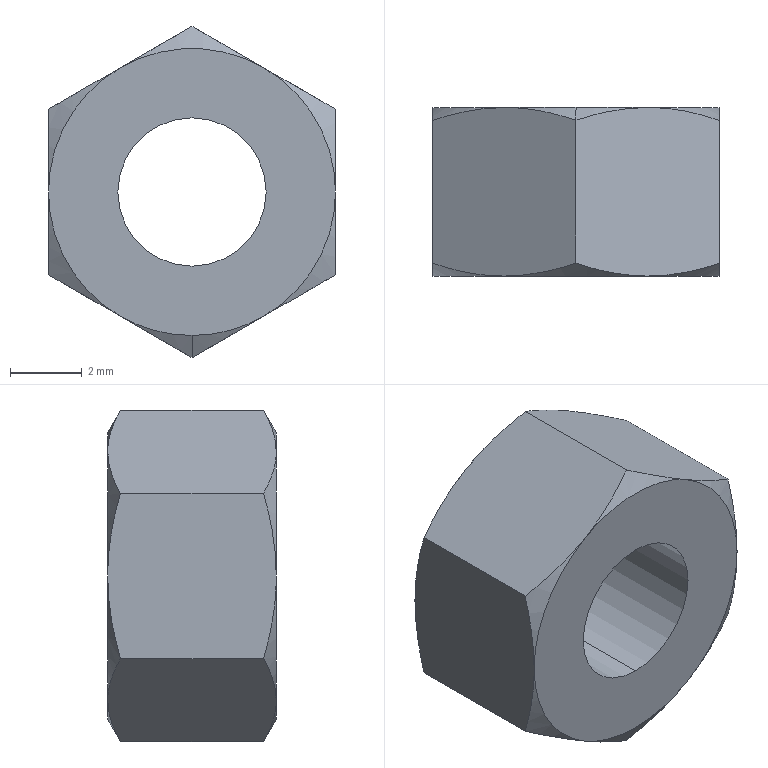Part | STEP file | 1 solid | 24 faces | box 8 x 4.7 x 9.238 mm | volume 196.298 mm3 | cone 14 | plane 8 | cylinder 2 | commonest cylinder face diameters 4.134 x2
STEP:
#1=CARTESIAN_POINT('',(2.,0.,-3.464));
#2=VERTEX_POINT('',#1);
#3=CARTESIAN_POINT('',(0.,0.,-4.));
#4=VERTEX_POINT('',#3);
#5=CARTESIAN_POINT('',(0.,0.,0.));
#6=DIRECTION('',(0.,1.,0.));
#7=DIRECTION('',(0.,0.,1.));
#8=AXIS2_PLACEMENT_3D('',#5,#6,#7);
#9=CIRCLE('',#8,4.);
#10=EDGE_CURVE('',#2,#4,#9,.T.);
#11=ORIENTED_EDGE('',*,*,#10,.T.);
#12=CARTESIAN_POINT('',(0.,0.3573,-4.619));
#13=VERTEX_POINT('',#12);
#14=CARTESIAN_POINT('',(0.,0.,-4.));
#15=DIRECTION('',(0.,0.5,-0.866));
#16=VECTOR('',#15,1000.);
#17=LINE('',#14,#16);
#18=EDGE_CURVE('',#4,#13,#17,.T.);
#19=ORIENTED_EDGE('',*,*,#18,.T.);
#20=CARTESIAN_POINT('',(0.,0.3573,-4.619));
#21=CARTESIAN_POINT('',(0.6543,0.1392,-4.241));
#22=CARTESIAN_POINT('',(1.319,0.,-3.858));
#23=CARTESIAN_POINT('',(2.,0.,-3.464));
#24=B_SPLINE_CURVE_WITH_KNOTS('',3,(#20,#21,#22,#23),.UNSPECIFIED.,.F.,.F.,(4,4),(0.000000238,0.002337),.UNSPECIFIED.);
#25=EDGE_CURVE('',#13,#2,#24,.T.);
#26=ORIENTED_EDGE('',*,*,#25,.T.);
#27=EDGE_LOOP('',(#11,#19,#26));
#28=FACE_OUTER_BOUND('',#27,.T.);
#29=CARTESIAN_POINT('',(0.,0.,0.));
#30=DIRECTION('',(0.,1.,0.));
#31=DIRECTION('',(0.,0.,-1.));
#32=AXIS2_PLACEMENT_3D('',#29,#30,#31);
#33=CONICAL_SURFACE('',#32,4.,1.047);
#34=ADVANCED_FACE('',(#28),#33,.T.);
#35=CARTESIAN_POINT('',(0.,4.7,4.));
#36=VERTEX_POINT('',#35);
#37=CARTESIAN_POINT('',(2.,4.7,3.464));
#38=VERTEX_POINT('',#37);
#39=CARTESIAN_POINT('',(0.,4.7,0.));
#40=DIRECTION('',(0.,1.,0.));
#41=DIRECTION('',(0.,0.,1.));
#42=AXIS2_PLACEMENT_3D('',#39,#40,#41);
#43=CIRCLE('',#42,4.);
#44=EDGE_CURVE('',#36,#38,#43,.T.);
#45=ORIENTED_EDGE('',*,*,#44,.F.);
#46=CARTESIAN_POINT('',(0.,4.343,4.619));
#47=VERTEX_POINT('',#46);
#48=CARTESIAN_POINT('',(0.,4.7,4.));
#49=DIRECTION('',(0.,-0.5,0.866));
#50=VECTOR('',#49,1000.);
#51=LINE('',#48,#50);
#52=EDGE_CURVE('',#36,#47,#51,.T.);
#53=ORIENTED_EDGE('',*,*,#52,.T.);
#54=CARTESIAN_POINT('',(0.,4.343,4.619));
#55=CARTESIAN_POINT('',(0.6543,4.561,4.241));
#56=CARTESIAN_POINT('',(1.319,4.7,3.858));
#57=CARTESIAN_POINT('',(2.,4.7,3.464));
#58=B_SPLINE_CURVE_WITH_KNOTS('',3,(#54,#55,#56,#57),.UNSPECIFIED.,.F.,.F.,(4,4),(0.000000238,0.002337),.UNSPECIFIED.);
#59=EDGE_CURVE('',#47,#38,#58,.T.);
#60=ORIENTED_EDGE('',*,*,#59,.T.);
#61=EDGE_LOOP('',(#45,#53,#60));
#62=FACE_OUTER_BOUND('',#61,.T.);
#63=CARTESIAN_POINT('',(0.,4.7,0.));
#64=DIRECTION('',(0.,-1.,0.));
#65=DIRECTION('',(0.,0.,1.));
#66=AXIS2_PLACEMENT_3D('',#63,#64,#65);
#67=CONICAL_SURFACE('',#66,4.,1.047);
#68=ADVANCED_FACE('',(#62),#67,.T.);
#69=CARTESIAN_POINT('',(0.,4.7,-2.067));
#70=VERTEX_POINT('',#69);
#71=CARTESIAN_POINT('',(0.,4.7,2.067));
#72=VERTEX_POINT('',#71);
#73=CARTESIAN_POINT('',(0.,4.7,0.));
#74=DIRECTION('',(0.,1.,0.));
#75=DIRECTION('',(0.,0.,1.));
#76=AXIS2_PLACEMENT_3D('',#73,#74,#75);
#77=CIRCLE('',#76,2.067);
#78=EDGE_CURVE('',#70,#72,#77,.T.);
#79=ORIENTED_EDGE('',*,*,#78,.T.);
#80=CARTESIAN_POINT('',(0.,0.,2.067));
#81=VERTEX_POINT('',#80);
#82=CARTESIAN_POINT('',(0.,4.7,2.067));
#83=DIRECTION('',(0.,-1.,0.));
#84=VECTOR('',#83,1000.);
#85=LINE('',#82,#84);
#86=EDGE_CURVE('',#72,#81,#85,.T.);
#87=ORIENTED_EDGE('',*,*,#86,.T.);
#88=CARTESIAN_POINT('',(0.,0.,-2.067));
#89=VERTEX_POINT('',#88);
#90=CARTESIAN_POINT('',(0.,0.,0.));
#91=DIRECTION('',(0.,1.,0.));
#92=DIRECTION('',(0.,0.,1.));
#93=AXIS2_PLACEMENT_3D('',#90,#91,#92);
#94=CIRCLE('',#93,2.067);
#95=EDGE_CURVE('',#89,#81,#94,.T.);
#96=ORIENTED_EDGE('',*,*,#95,.F.);
#97=CARTESIAN_POINT('',(0.,4.7,-2.067));
#98=DIRECTION('',(0.,-1.,0.));
#99=VECTOR('',#98,1000.);
#100=LINE('',#97,#99);
#101=EDGE_CURVE('',#70,#89,#100,.T.);
#102=ORIENTED_EDGE('',*,*,#101,.F.);
#103=EDGE_LOOP('',(#79,#87,#96,#102));
#104=FACE_OUTER_BOUND('',#103,.T.);
#105=CARTESIAN_POINT('',(0.,4.7,0.));
#106=DIRECTION('',(0.,-1.,0.));
#107=DIRECTION('',(0.,0.,-1.));
#108=AXIS2_PLACEMENT_3D('',#105,#106,#107);
#109=CYLINDRICAL_SURFACE('',#108,2.067);
#110=ADVANCED_FACE('',(#104),#109,.F.);
#111=CARTESIAN_POINT('',(-4.,0.3573,-2.309));
#112=VERTEX_POINT('',#111);
#113=CARTESIAN_POINT('',(-2.,0.,-3.464));
#114=VERTEX_POINT('',#113);
#115=CARTESIAN_POINT('',(-4.,0.3573,-2.309));
#116=CARTESIAN_POINT('',(-3.346,0.1392,-2.687));
#117=CARTESIAN_POINT('',(-2.681,0.,-3.071));
#118=CARTESIAN_POINT('',(-2.,0.,-3.464));
#119=B_SPLINE_CURVE_WITH_KNOTS('',3,(#115,#116,#117,#118),.UNSPECIFIED.,.F.,.F.,(4,4),(0.000000238,0.002337),.UNSPECIFIED.);
#120=EDGE_CURVE('',#112,#114,#119,.T.);
#121=ORIENTED_EDGE('',*,*,#120,.F.);
#122=CARTESIAN_POINT('',(-4.,4.343,-2.309));
#123=VERTEX_POINT('',#122);
#124=CARTESIAN_POINT('',(-4.,4.7,-2.309));
#125=DIRECTION('',(0.,-1.,0.));
#126=VECTOR('',#125,1000.);
#127=LINE('',#124,#126);
#128=EDGE_CURVE('',#123,#112,#127,.T.);
#129=ORIENTED_EDGE('',*,*,#128,.F.);
#130=CARTESIAN_POINT('',(-2.,4.7,-3.464));
#131=VERTEX_POINT('',#130);
#132=CARTESIAN_POINT('',(-2.,4.7,-3.464));
#133=CARTESIAN_POINT('',(-2.339,4.7,-3.268));
#134=CARTESIAN_POINT('',(-2.678,4.666,-3.072));
#135=CARTESIAN_POINT('',(-3.345,4.541,-2.688));
#136=CARTESIAN_POINT('',(-3.674,4.452,-2.498));
#137=CARTESIAN_POINT('',(-4.,4.343,-2.309));
#138=B_SPLINE_CURVE_WITH_KNOTS('',3,(#132,#133,#134,#135,#136,#137),.UNSPECIFIED.,.F.,.F.,(4,2,4),(0.002337,0.003501,0.004665),.UNSPECIFIED.);
#139=EDGE_CURVE('',#131,#123,#138,.T.);
#140=ORIENTED_EDGE('',*,*,#139,.F.);
#141=CARTESIAN_POINT('',(0.,4.343,-4.619));
#142=VERTEX_POINT('',#141);
#143=CARTESIAN_POINT('',(0.,4.343,-4.619));
#144=CARTESIAN_POINT('',(-0.6543,4.561,-4.241));
#145=CARTESIAN_POINT('',(-1.319,4.7,-3.858));
#146=CARTESIAN_POINT('',(-2.,4.7,-3.464));
#147=B_SPLINE_CURVE_WITH_KNOTS('',3,(#143,#144,#145,#146),.UNSPECIFIED.,.F.,.F.,(4,4),(0.000000238,0.002337),.UNSPECIFIED.);
#148=EDGE_CURVE('',#142,#131,#147,.T.);
#149=ORIENTED_EDGE('',*,*,#148,.F.);
#150=CARTESIAN_POINT('',(0.,4.7,-4.619));
#151=DIRECTION('',(0.,-1.,0.));
#152=VECTOR('',#151,1000.);
#153=LINE('',#150,#152);
#154=EDGE_CURVE('',#142,#13,#153,.T.);
#155=ORIENTED_EDGE('',*,*,#154,.T.);
#156=CARTESIAN_POINT('',(-2.,0.,-3.464));
#157=CARTESIAN_POINT('',(-1.661,0.,-3.66));
#158=CARTESIAN_POINT('',(-1.322,0.03421,-3.856));
#159=CARTESIAN_POINT('',(-0.6554,0.1587,-4.24));
#160=CARTESIAN_POINT('',(-0.3264,0.2485,-4.43));
#161=CARTESIAN_POINT('',(0.,0.3573,-4.619));
#162=B_SPLINE_CURVE_WITH_KNOTS('',3,(#156,#157,#158,#159,#160,#161),.UNSPECIFIED.,.F.,.F.,(4,2,4),(0.002337,0.003501,0.004665),.UNSPECIFIED.);
#163=EDGE_CURVE('',#114,#13,#162,.T.);
#164=ORIENTED_EDGE('',*,*,#163,.F.);
#165=EDGE_LOOP('',(#121,#129,#140,#149,#155,#164));
#166=FACE_OUTER_BOUND('',#165,.T.);
#167=CARTESIAN_POINT('',(0.,4.7,-4.619));
#168=DIRECTION('',(0.5,0.,0.866));
#169=DIRECTION('',(0.866,0.,-0.5));
#170=AXIS2_PLACEMENT_3D('',#167,#168,#169);
#171=PLANE('',#170);
#172=ADVANCED_FACE('',(#166),#171,.F.);
#173=CARTESIAN_POINT('',(-4.,0.3573,2.309));
#174=VERTEX_POINT('',#173);
#175=CARTESIAN_POINT('',(-4.,0.,0.));
#176=VERTEX_POINT('',#175);
#177=CARTESIAN_POINT('',(-4.,0.3573,2.309));
#178=CARTESIAN_POINT('',(-4.,0.2494,1.936));
#179=CARTESIAN_POINT('',(-4.,0.1597,1.558));
#180=CARTESIAN_POINT('',(-4.,0.03454,0.7868));
#181=CARTESIAN_POINT('',(-4.,0.,0.3908));
#182=CARTESIAN_POINT('',(-4.,0.,0.));
#183=B_SPLINE_CURVE_WITH_KNOTS('',3,(#177,#178,#179,#180,#181,#182),.UNSPECIFIED.,.F.,.F.,(4,2,4),(0.0131,0.01427,0.01544),.UNSPECIFIED.);
#184=EDGE_CURVE('',#174,#176,#183,.T.);
#185=ORIENTED_EDGE('',*,*,#184,.F.);
#186=CARTESIAN_POINT('',(-4.,4.343,2.309));
#187=VERTEX_POINT('',#186);
#188=CARTESIAN_POINT('',(-4.,4.7,2.309));
#189=DIRECTION('',(0.,-1.,0.));
#190=VECTOR('',#189,1000.);
#191=LINE('',#188,#190);
#192=EDGE_CURVE('',#187,#174,#191,.T.);
#193=ORIENTED_EDGE('',*,*,#192,.F.);
#194=CARTESIAN_POINT('',(-4.,4.7,0.));
#195=VERTEX_POINT('',#194);
#196=CARTESIAN_POINT('',(-4.,4.7,0.));
#197=CARTESIAN_POINT('',(-4.,4.7,0.3908));
#198=CARTESIAN_POINT('',(-4.,4.665,0.7868));
#199=CARTESIAN_POINT('',(-4.,4.54,1.558));
#200=CARTESIAN_POINT('',(-4.,4.451,1.936));
#201=CARTESIAN_POINT('',(-4.,4.343,2.309));
#202=B_SPLINE_CURVE_WITH_KNOTS('',3,(#196,#197,#198,#199,#200,#201),.UNSPECIFIED.,.F.,.F.,(4,2,4),(0.006565,0.007734,0.008904),.UNSPECIFIED.);
#203=EDGE_CURVE('',#195,#187,#202,.T.);
#204=ORIENTED_EDGE('',*,*,#203,.F.);
#205=CARTESIAN_POINT('',(-4.,4.343,-2.309));
#206=CARTESIAN_POINT('',(-4.,4.451,-1.933));
#207=CARTESIAN_POINT('',(-4.,4.542,-1.549));
#208=CARTESIAN_POINT('',(-4.,4.666,-0.7783));
#209=CARTESIAN_POINT('',(-4.,4.7,-0.3906));
#210=CARTESIAN_POINT('',(-4.,4.7,0.));
#211=B_SPLINE_CURVE_WITH_KNOTS('',3,(#205,#206,#207,#208,#209,#210),.UNSPECIFIED.,.F.,.F.,(4,2,4),(0.004227,0.005396,0.006565),.UNSPECIFIED.);
#212=EDGE_CURVE('',#123,#195,#211,.T.);
#213=ORIENTED_EDGE('',*,*,#212,.F.);
#214=ORIENTED_EDGE('',*,*,#128,.T.);
#215=CARTESIAN_POINT('',(-4.,0.,0.));
#216=CARTESIAN_POINT('',(-4.,0.,-0.3906));
#217=CARTESIAN_POINT('',(-4.,0.03359,-0.7783));
#218=CARTESIAN_POINT('',(-4.,0.1579,-1.549));
#219=CARTESIAN_POINT('',(-4.,0.2487,-1.933));
#220=CARTESIAN_POINT('',(-4.,0.3573,-2.309));
#221=B_SPLINE_CURVE_WITH_KNOTS('',3,(#215,#216,#217,#218,#219,#220),.UNSPECIFIED.,.F.,.F.,(4,2,4),(0.01544,0.01661,0.01777),.UNSPECIFIED.);
#222=EDGE_CURVE('',#176,#112,#221,.T.);
#223=ORIENTED_EDGE('',*,*,#222,.F.);
#224=EDGE_LOOP('',(#185,#193,#204,#213,#214,#223));
#225=FACE_OUTER_BOUND('',#224,.T.);
#226=CARTESIAN_POINT('',(-4.,4.7,-2.309));
#227=DIRECTION('',(1.,0.,0.));
#228=DIRECTION('',(0.,0.,-1.));
#229=AXIS2_PLACEMENT_3D('',#226,#227,#228);
#230=PLANE('',#229);
#231=ADVANCED_FACE('',(#225),#230,.F.);
#232=CARTESIAN_POINT('',(0.,0.3573,4.619));
#233=VERTEX_POINT('',#232);
#234=CARTESIAN_POINT('',(-2.,0.,3.464));
#235=VERTEX_POINT('',#234);
#236=CARTESIAN_POINT('',(0.,0.3573,4.619));
#237=CARTESIAN_POINT('',(-0.6543,0.1392,4.241));
#238=CARTESIAN_POINT('',(-1.319,0.,3.858));
#239=CARTESIAN_POINT('',(-2.,0.,3.464));
#240=B_SPLINE_CURVE_WITH_KNOTS('',3,(#236,#237,#238,#239),.UNSPECIFIED.,.F.,.F.,(4,4),(0.000000238,0.002337),.UNSPECIFIED.);
#241=EDGE_CURVE('',#233,#235,#240,.T.);
#242=ORIENTED_EDGE('',*,*,#241,.F.);
#243=CARTESIAN_POINT('',(0.,4.7,4.619));
#244=DIRECTION('',(0.,-1.,0.));
#245=VECTOR('',#244,1000.);
#246=LINE('',#243,#245);
#247=EDGE_CURVE('',#47,#233,#246,.T.);
#248=ORIENTED_EDGE('',*,*,#247,.F.);
#249=CARTESIAN_POINT('',(-2.,4.7,3.464));
#250=VERTEX_POINT('',#249);
#251=CARTESIAN_POINT('',(-2.,4.7,3.464));
#252=CARTESIAN_POINT('',(-1.661,4.7,3.66));
#253=CARTESIAN_POINT('',(-1.322,4.666,3.856));
#254=CARTESIAN_POINT('',(-0.6554,4.541,4.24));
#255=CARTESIAN_POINT('',(-0.3264,4.452,4.43));
#256=CARTESIAN_POINT('',(0.,4.343,4.619));
#257=B_SPLINE_CURVE_WITH_KNOTS('',3,(#251,#252,#253,#254,#255,#256),.UNSPECIFIED.,.F.,.F.,(4,2,4),(0.002337,0.003501,0.004665),.UNSPECIFIED.);
#258=EDGE_CURVE('',#250,#47,#257,.T.);
#259=ORIENTED_EDGE('',*,*,#258,.F.);
#260=CARTESIAN_POINT('',(-4.,4.343,2.309));
#261=CARTESIAN_POINT('',(-3.346,4.561,2.687));
#262=CARTESIAN_POINT('',(-2.681,4.7,3.071));
#263=CARTESIAN_POINT('',(-2.,4.7,3.464));
#264=B_SPLINE_CURVE_WITH_KNOTS('',3,(#260,#261,#262,#263),.UNSPECIFIED.,.F.,.F.,(4,4),(0.000000238,0.002337),.UNSPECIFIED.);
#265=EDGE_CURVE('',#187,#250,#264,.T.);
#266=ORIENTED_EDGE('',*,*,#265,.F.);
#267=ORIENTED_EDGE('',*,*,#192,.T.);
#268=CARTESIAN_POINT('',(-2.,0.,3.464));
#269=CARTESIAN_POINT('',(-2.339,0.,3.268));
#270=CARTESIAN_POINT('',(-2.678,0.03421,3.072));
#271=CARTESIAN_POINT('',(-3.345,0.1587,2.688));
#272=CARTESIAN_POINT('',(-3.674,0.2485,2.498));
#273=CARTESIAN_POINT('',(-4.,0.3573,2.309));
#274=B_SPLINE_CURVE_WITH_KNOTS('',3,(#268,#269,#270,#271,#272,#273),.UNSPECIFIED.,.F.,.F.,(4,2,4),(0.002337,0.003501,0.004665),.UNSPECIFIED.);
#275=EDGE_CURVE('',#235,#174,#274,.T.);
#276=ORIENTED_EDGE('',*,*,#275,.F.);
#277=EDGE_LOOP('',(#242,#248,#259,#266,#267,#276));
#278=FACE_OUTER_BOUND('',#277,.T.);
#279=CARTESIAN_POINT('',(-4.,4.7,2.309));
#280=DIRECTION('',(0.5,0.,-0.866));
#281=DIRECTION('',(-0.866,0.,-0.5));
#282=AXIS2_PLACEMENT_3D('',#279,#280,#281);
#283=PLANE('',#282);
#284=ADVANCED_FACE('',(#278),#283,.F.);
#285=CARTESIAN_POINT('',(4.,0.3573,2.309));
#286=VERTEX_POINT('',#285);
#287=CARTESIAN_POINT('',(2.,0.,3.464));
#288=VERTEX_POINT('',#287);
#289=CARTESIAN_POINT('',(4.,0.3573,2.309));
#290=CARTESIAN_POINT('',(3.346,0.1392,2.687));
#291=CARTESIAN_POINT('',(2.681,0.,3.071));
#292=CARTESIAN_POINT('',(2.,0.,3.464));
#293=B_SPLINE_CURVE_WITH_KNOTS('',3,(#289,#290,#291,#292),.UNSPECIFIED.,.F.,.F.,(4,4),(0.000000238,0.002337),.UNSPECIFIED.);
#294=EDGE_CURVE('',#286,#288,#293,.T.);
#295=ORIENTED_EDGE('',*,*,#294,.F.);
#296=CARTESIAN_POINT('',(4.,4.343,2.309));
#297=VERTEX_POINT('',#296);
#298=CARTESIAN_POINT('',(4.,4.7,2.309));
#299=DIRECTION('',(0.,-1.,0.));
#300=VECTOR('',#299,1000.);
#301=LINE('',#298,#300);
#302=EDGE_CURVE('',#297,#286,#301,.T.);
#303=ORIENTED_EDGE('',*,*,#302,.F.);
#304=CARTESIAN_POINT('',(2.,4.7,3.464));
#305=CARTESIAN_POINT('',(2.339,4.7,3.268));
#306=CARTESIAN_POINT('',(2.678,4.666,3.072));
#307=CARTESIAN_POINT('',(3.345,4.541,2.688));
#308=CARTESIAN_POINT('',(3.674,4.452,2.498));
#309=CARTESIAN_POINT('',(4.,4.343,2.309));
#310=B_SPLINE_CURVE_WITH_KNOTS('',3,(#304,#305,#306,#307,#308,#309),.UNSPECIFIED.,.F.,.F.,(4,2,4),(0.002337,0.003501,0.004665),.UNSPECIFIED.);
#311=EDGE_CURVE('',#38,#297,#310,.T.);
#312=ORIENTED_EDGE('',*,*,#311,.F.);
#313=ORIENTED_EDGE('',*,*,#59,.F.);
#314=ORIENTED_EDGE('',*,*,#247,.T.);
#315=CARTESIAN_POINT('',(2.,0.,3.464));
#316=CARTESIAN_POINT('',(1.661,0.,3.66));
#317=CARTESIAN_POINT('',(1.322,0.03421,3.856));
#318=CARTESIAN_POINT('',(0.6554,0.1587,4.24));
#319=CARTESIAN_POINT('',(0.3264,0.2485,4.43));
#320=CARTESIAN_POINT('',(0.,0.3573,4.619));
#321=B_SPLINE_CURVE_WITH_KNOTS('',3,(#315,#316,#317,#318,#319,#320),.UNSPECIFIED.,.F.,.F.,(4,2,4),(0.002337,0.003501,0.004665),.UNSPECIFIED.);
#322=EDGE_CURVE('',#288,#233,#321,.T.);
#323=ORIENTED_EDGE('',*,*,#322,.F.);
#324=EDGE_LOOP('',(#295,#303,#312,#313,#314,#323));
#325=FACE_OUTER_BOUND('',#324,.T.);
#326=CARTESIAN_POINT('',(0.,4.7,4.619));
#327=DIRECTION('',(-0.5,0.,-0.866));
#328=DIRECTION('',(-0.866,0.,0.5));
#329=AXIS2_PLACEMENT_3D('',#326,#327,#328);
#330=PLANE('',#329);
#331=ADVANCED_FACE('',(#325),#330,.F.);
#332=CARTESIAN_POINT('',(4.,0.3573,-2.309));
#333=VERTEX_POINT('',#332);
#334=CARTESIAN_POINT('',(4.,0.,0.));
#335=VERTEX_POINT('',#334);
#336=CARTESIAN_POINT('',(4.,0.3573,-2.309));
#337=CARTESIAN_POINT('',(4.,0.2487,-1.933));
#338=CARTESIAN_POINT('',(4.,0.1579,-1.549));
#339=CARTESIAN_POINT('',(4.,0.03359,-0.7783));
#340=CARTESIAN_POINT('',(4.,0.,-0.3906));
#341=CARTESIAN_POINT('',(4.,0.,0.));
#342=B_SPLINE_CURVE_WITH_KNOTS('',3,(#336,#337,#338,#339,#340,#341),.UNSPECIFIED.,.F.,.F.,(4,2,4),(0.004227,0.005396,0.006565),.UNSPECIFIED.);
#343=EDGE_CURVE('',#333,#335,#342,.T.);
#344=ORIENTED_EDGE('',*,*,#343,.F.);
#345=CARTESIAN_POINT('',(4.,4.343,-2.309));
#346=VERTEX_POINT('',#345);
#347=CARTESIAN_POINT('',(4.,4.7,-2.309));
#348=DIRECTION('',(0.,-1.,0.));
#349=VECTOR('',#348,1000.);
#350=LINE('',#347,#349);
#351=EDGE_CURVE('',#346,#333,#350,.T.);
#352=ORIENTED_EDGE('',*,*,#351,.F.);
#353=CARTESIAN_POINT('',(4.,4.7,0.));
#354=VERTEX_POINT('',#353);
#355=CARTESIAN_POINT('',(4.,4.7,0.));
#356=CARTESIAN_POINT('',(4.,4.7,-0.3906));
#357=CARTESIAN_POINT('',(4.,4.666,-0.7783));
#358=CARTESIAN_POINT('',(4.,4.542,-1.549));
#359=CARTESIAN_POINT('',(4.,4.451,-1.933));
#360=CARTESIAN_POINT('',(4.,4.343,-2.309));
#361=B_SPLINE_CURVE_WITH_KNOTS('',3,(#355,#356,#357,#358,#359,#360),.UNSPECIFIED.,.F.,.F.,(4,2,4),(0.01544,0.01661,0.01777),.UNSPECIFIED.);
#362=EDGE_CURVE('',#354,#346,#361,.T.);
#363=ORIENTED_EDGE('',*,*,#362,.F.);
#364=CARTESIAN_POINT('',(4.,4.343,2.309));
#365=CARTESIAN_POINT('',(4.,4.451,1.936));
#366=CARTESIAN_POINT('',(4.,4.54,1.558));
#367=CARTESIAN_POINT('',(4.,4.665,0.7868));
#368=CARTESIAN_POINT('',(4.,4.7,0.3908));
#369=CARTESIAN_POINT('',(4.,4.7,0.));
#370=B_SPLINE_CURVE_WITH_KNOTS('',3,(#364,#365,#366,#367,#368,#369),.UNSPECIFIED.,.F.,.F.,(4,2,4),(0.0131,0.01427,0.01544),.UNSPECIFIED.);
#371=EDGE_CURVE('',#297,#354,#370,.T.);
#372=ORIENTED_EDGE('',*,*,#371,.F.);
#373=ORIENTED_EDGE('',*,*,#302,.T.);
#374=CARTESIAN_POINT('',(4.,0.,0.));
#375=CARTESIAN_POINT('',(4.,0.,0.3908));
#376=CARTESIAN_POINT('',(4.,0.03454,0.7868));
#377=CARTESIAN_POINT('',(4.,0.1597,1.558));
#378=CARTESIAN_POINT('',(4.,0.2494,1.936));
#379=CARTESIAN_POINT('',(4.,0.3573,2.309));
#380=B_SPLINE_CURVE_WITH_KNOTS('',3,(#374,#375,#376,#377,#378,#379),.UNSPECIFIED.,.F.,.F.,(4,2,4),(0.006565,0.007734,0.008904),.UNSPECIFIED.);
#381=EDGE_CURVE('',#335,#286,#380,.T.);
#382=ORIENTED_EDGE('',*,*,#381,.F.);
#383=EDGE_LOOP('',(#344,#352,#363,#372,#373,#382));
#384=FACE_OUTER_BOUND('',#383,.T.);
#385=CARTESIAN_POINT('',(4.,4.7,2.309));
#386=DIRECTION('',(-1.,0.,0.));
#387=DIRECTION('',(0.,0.,1.));
#388=AXIS2_PLACEMENT_3D('',#385,#386,#387);
#389=PLANE('',#388);
#390=ADVANCED_FACE('',(#384),#389,.F.);
#391=ORIENTED_EDGE('',*,*,#25,.F.);
#392=ORIENTED_EDGE('',*,*,#154,.F.);
#393=CARTESIAN_POINT('',(2.,4.7,-3.464));
#394=VERTEX_POINT('',#393);
#395=CARTESIAN_POINT('',(2.,4.7,-3.464));
#396=CARTESIAN_POINT('',(1.661,4.7,-3.66));
#397=CARTESIAN_POINT('',(1.322,4.666,-3.856));
#398=CARTESIAN_POINT('',(0.6554,4.541,-4.24));
#399=CARTESIAN_POINT('',(0.3264,4.452,-4.43));
#400=CARTESIAN_POINT('',(0.,4.343,-4.619));
#401=B_SPLINE_CURVE_WITH_KNOTS('',3,(#395,#396,#397,#398,#399,#400),.UNSPECIFIED.,.F.,.F.,(4,2,4),(0.002337,0.003501,0.004665),.UNSPECIFIED.);
#402=EDGE_CURVE('',#394,#142,#401,.T.);
#403=ORIENTED_EDGE('',*,*,#402,.F.);
#404=CARTESIAN_POINT('',(4.,4.343,-2.309));
#405=CARTESIAN_POINT('',(3.346,4.561,-2.687));
#406=CARTESIAN_POINT('',(2.681,4.7,-3.071));
#407=CARTESIAN_POINT('',(2.,4.7,-3.464));
#408=B_SPLINE_CURVE_WITH_KNOTS('',3,(#404,#405,#406,#407),.UNSPECIFIED.,.F.,.F.,(4,4),(0.000000238,0.002337),.UNSPECIFIED.);
#409=EDGE_CURVE('',#346,#394,#408,.T.);
#410=ORIENTED_EDGE('',*,*,#409,.F.);
#411=ORIENTED_EDGE('',*,*,#351,.T.);
#412=CARTESIAN_POINT('',(2.,0.,-3.464));
#413=CARTESIAN_POINT('',(2.339,0.,-3.268));
#414=CARTESIAN_POINT('',(2.678,0.03421,-3.072));
#415=CARTESIAN_POINT('',(3.345,0.1587,-2.688));
#416=CARTESIAN_POINT('',(3.674,0.2485,-2.498));
#417=CARTESIAN_POINT('',(4.,0.3573,-2.309));
#418=B_SPLINE_CURVE_WITH_KNOTS('',3,(#412,#413,#414,#415,#416,#417),.UNSPECIFIED.,.F.,.F.,(4,2,4),(0.002337,0.003501,0.004665),.UNSPECIFIED.);
#419=EDGE_CURVE('',#2,#333,#418,.T.);
#420=ORIENTED_EDGE('',*,*,#419,.F.);
#421=EDGE_LOOP('',(#391,#392,#403,#410,#411,#420));
#422=FACE_OUTER_BOUND('',#421,.T.);
#423=CARTESIAN_POINT('',(4.,4.7,-2.309));
#424=DIRECTION('',(-0.5,0.,0.866));
#425=DIRECTION('',(0.866,0.,0.5));
#426=AXIS2_PLACEMENT_3D('',#423,#424,#425);
#427=PLANE('',#426);
#428=ADVANCED_FACE('',(#422),#427,.F.);
#429=ORIENTED_EDGE('',*,*,#95,.T.);
#430=CARTESIAN_POINT('',(0.,0.,0.));
#431=DIRECTION('',(0.,1.,0.));
#432=DIRECTION('',(0.,0.,1.));
#433=AXIS2_PLACEMENT_3D('',#430,#431,#432);
#434=CIRCLE('',#433,2.067);
#435=EDGE_CURVE('',#81,#89,#434,.T.);
#436=ORIENTED_EDGE('',*,*,#435,.T.);
#437=EDGE_LOOP('',(#429,#436));
#438=FACE_BOUND('',#437,.T.);
#439=CARTESIAN_POINT('',(0.,0.,0.));
#440=DIRECTION('',(0.,1.,0.));
#441=DIRECTION('',(0.,0.,1.));
#442=AXIS2_PLACEMENT_3D('',#439,#440,#441);
#443=CIRCLE('',#442,4.);
#444=EDGE_CURVE('',#288,#335,#443,.T.);
#445=ORIENTED_EDGE('',*,*,#444,.F.);
#446=CARTESIAN_POINT('',(0.,0.,0.));
#447=DIRECTION('',(0.,1.,0.));
#448=DIRECTION('',(0.,0.,1.));
#449=AXIS2_PLACEMENT_3D('',#446,#447,#448);
#450=CIRCLE('',#449,4.);
#451=EDGE_CURVE('',#235,#288,#450,.T.);
#452=ORIENTED_EDGE('',*,*,#451,.F.);
#453=CARTESIAN_POINT('',(0.,0.,0.));
#454=DIRECTION('',(0.,1.,0.));
#455=DIRECTION('',(0.,0.,1.));
#456=AXIS2_PLACEMENT_3D('',#453,#454,#455);
#457=CIRCLE('',#456,4.);
#458=EDGE_CURVE('',#176,#235,#457,.T.);
#459=ORIENTED_EDGE('',*,*,#458,.F.);
#460=CARTESIAN_POINT('',(0.,0.,0.));
#461=DIRECTION('',(0.,1.,0.));
#462=DIRECTION('',(0.,0.,1.));
#463=AXIS2_PLACEMENT_3D('',#460,#461,#462);
#464=CIRCLE('',#463,4.);
#465=EDGE_CURVE('',#114,#176,#464,.T.);
#466=ORIENTED_EDGE('',*,*,#465,.F.);
#467=CARTESIAN_POINT('',(0.,0.,0.));
#468=DIRECTION('',(0.,1.,0.));
#469=DIRECTION('',(0.,0.,1.));
#470=AXIS2_PLACEMENT_3D('',#467,#468,#469);
#471=CIRCLE('',#470,4.);
#472=EDGE_CURVE('',#4,#114,#471,.T.);
#473=ORIENTED_EDGE('',*,*,#472,.F.);
#474=ORIENTED_EDGE('',*,*,#10,.F.);
#475=CARTESIAN_POINT('',(0.,0.,0.));
#476=DIRECTION('',(0.,-1.,0.));
#477=DIRECTION('',(0.,0.,-1.));
#478=AXIS2_PLACEMENT_3D('',#475,#476,#477);
#479=CIRCLE('',#478,4.);
#480=EDGE_CURVE('',#2,#335,#479,.T.);
#481=ORIENTED_EDGE('',*,*,#480,.T.);
#482=EDGE_LOOP('',(#445,#452,#459,#466,#473,#474,#481));
#483=FACE_OUTER_BOUND('',#482,.T.);
#484=CARTESIAN_POINT('',(0.,0.,0.));
#485=DIRECTION('',(0.,1.,0.));
#486=DIRECTION('',(0.,0.,1.));
#487=AXIS2_PLACEMENT_3D('',#484,#485,#486);
#488=PLANE('',#487);
#489=ADVANCED_FACE('',(#438,#483),#488,.F.);
#490=ORIENTED_EDGE('',*,*,#78,.F.);
#491=CARTESIAN_POINT('',(0.,4.7,0.));
#492=DIRECTION('',(0.,1.,0.));
#493=DIRECTION('',(0.,0.,1.));
#494=AXIS2_PLACEMENT_3D('',#491,#492,#493);
#495=CIRCLE('',#494,2.067);
#496=EDGE_CURVE('',#72,#70,#495,.T.);
#497=ORIENTED_EDGE('',*,*,#496,.F.);
#498=EDGE_LOOP('',(#490,#497));
#499=FACE_BOUND('',#498,.T.);
#500=CARTESIAN_POINT('',(0.,4.7,0.));
#501=DIRECTION('',(0.,1.,0.));
#502=DIRECTION('',(0.,0.,1.));
#503=AXIS2_PLACEMENT_3D('',#500,#501,#502);
#504=CIRCLE('',#503,4.);
#505=EDGE_CURVE('',#250,#36,#504,.T.);
#506=ORIENTED_EDGE('',*,*,#505,.T.);
#507=ORIENTED_EDGE('',*,*,#44,.T.);
#508=CARTESIAN_POINT('',(0.,4.7,0.));
#509=DIRECTION('',(0.,1.,0.));
#510=DIRECTION('',(0.,0.,1.));
#511=AXIS2_PLACEMENT_3D('',#508,#509,#510);
#512=CIRCLE('',#511,4.);
#513=EDGE_CURVE('',#38,#354,#512,.T.);
#514=ORIENTED_EDGE('',*,*,#513,.T.);
#515=CARTESIAN_POINT('',(0.,4.7,0.));
#516=DIRECTION('',(0.,1.,0.));
#517=DIRECTION('',(0.,0.,1.));
#518=AXIS2_PLACEMENT_3D('',#515,#516,#517);
#519=CIRCLE('',#518,4.);
#520=EDGE_CURVE('',#354,#394,#519,.T.);
#521=ORIENTED_EDGE('',*,*,#520,.T.);
#522=CARTESIAN_POINT('',(0.,4.7,0.));
#523=DIRECTION('',(0.,1.,0.));
#524=DIRECTION('',(0.,0.,1.));
#525=AXIS2_PLACEMENT_3D('',#522,#523,#524);
#526=CIRCLE('',#525,4.);
#527=EDGE_CURVE('',#394,#131,#526,.T.);
#528=ORIENTED_EDGE('',*,*,#527,.T.);
#529=CARTESIAN_POINT('',(0.,4.7,0.));
#530=DIRECTION('',(0.,1.,0.));
#531=DIRECTION('',(0.,0.,1.));
#532=AXIS2_PLACEMENT_3D('',#529,#530,#531);
#533=CIRCLE('',#532,4.);
#534=EDGE_CURVE('',#131,#195,#533,.T.);
#535=ORIENTED_EDGE('',*,*,#534,.T.);
#536=CARTESIAN_POINT('',(0.,4.7,0.));
#537=DIRECTION('',(0.,1.,0.));
#538=DIRECTION('',(0.,0.,1.));
#539=AXIS2_PLACEMENT_3D('',#536,#537,#538);
#540=CIRCLE('',#539,4.);
#541=EDGE_CURVE('',#195,#250,#540,.T.);
#542=ORIENTED_EDGE('',*,*,#541,.T.);
#543=EDGE_LOOP('',(#506,#507,#514,#521,#528,#535,#542));
#544=FACE_OUTER_BOUND('',#543,.T.);
#545=CARTESIAN_POINT('',(0.,4.7,0.));
#546=DIRECTION('',(0.,1.,0.));
#547=DIRECTION('',(0.,0.,1.));
#548=AXIS2_PLACEMENT_3D('',#545,#546,#547);
#549=PLANE('',#548);
#550=ADVANCED_FACE('',(#499,#544),#549,.T.);
#551=ORIENTED_EDGE('',*,*,#86,.F.);
#552=ORIENTED_EDGE('',*,*,#496,.T.);
#553=ORIENTED_EDGE('',*,*,#101,.T.);
#554=ORIENTED_EDGE('',*,*,#435,.F.);
#555=EDGE_LOOP('',(#551,#552,#553,#554));
#556=FACE_OUTER_BOUND('',#555,.T.);
#557=CARTESIAN_POINT('',(0.,4.7,0.));
#558=DIRECTION('',(0.,-1.,0.));
#559=DIRECTION('',(0.,0.,-1.));
#560=AXIS2_PLACEMENT_3D('',#557,#558,#559);
#561=CYLINDRICAL_SURFACE('',#560,2.067);
#562=ADVANCED_FACE('',(#556),#561,.F.);
#563=ORIENTED_EDGE('',*,*,#148,.T.);
#564=ORIENTED_EDGE('',*,*,#527,.F.);
#565=ORIENTED_EDGE('',*,*,#402,.T.);
#566=EDGE_LOOP('',(#563,#564,#565));
#567=FACE_OUTER_BOUND('',#566,.T.);
#568=CARTESIAN_POINT('',(0.,4.7,0.));
#569=DIRECTION('',(0.,-1.,0.));
#570=DIRECTION('',(0.,0.,1.));
#571=AXIS2_PLACEMENT_3D('',#568,#569,#570);
#572=CONICAL_SURFACE('',#571,4.,1.047);
#573=ADVANCED_FACE('',(#567),#572,.T.);
#574=ORIENTED_EDGE('',*,*,#362,.T.);
#575=ORIENTED_EDGE('',*,*,#409,.T.);
#576=ORIENTED_EDGE('',*,*,#520,.F.);
#577=EDGE_LOOP('',(#574,#575,#576));
#578=FACE_OUTER_BOUND('',#577,.T.);
#579=CARTESIAN_POINT('',(0.,4.7,0.));
#580=DIRECTION('',(0.,-1.,0.));
#581=DIRECTION('',(0.,0.,1.));
#582=AXIS2_PLACEMENT_3D('',#579,#580,#581);
#583=CONICAL_SURFACE('',#582,4.,1.047);
#584=ADVANCED_FACE('',(#578),#583,.T.);
#585=ORIENTED_EDGE('',*,*,#311,.T.);
#586=ORIENTED_EDGE('',*,*,#371,.T.);
#587=ORIENTED_EDGE('',*,*,#513,.F.);
#588=EDGE_LOOP('',(#585,#586,#587));
#589=FACE_OUTER_BOUND('',#588,.T.);
#590=CARTESIAN_POINT('',(0.,4.7,0.));
#591=DIRECTION('',(0.,-1.,0.));
#592=DIRECTION('',(0.,0.,1.));
#593=AXIS2_PLACEMENT_3D('',#590,#591,#592);
#594=CONICAL_SURFACE('',#593,4.,1.047);
#595=ADVANCED_FACE('',(#589),#594,.T.);
#596=ORIENTED_EDGE('',*,*,#52,.F.);
#597=ORIENTED_EDGE('',*,*,#505,.F.);
#598=ORIENTED_EDGE('',*,*,#258,.T.);
#599=EDGE_LOOP('',(#596,#597,#598));
#600=FACE_OUTER_BOUND('',#599,.T.);
#601=CARTESIAN_POINT('',(0.,4.7,0.));
#602=DIRECTION('',(0.,-1.,0.));
#603=DIRECTION('',(0.,0.,1.));
#604=AXIS2_PLACEMENT_3D('',#601,#602,#603);
#605=CONICAL_SURFACE('',#604,4.,1.047);
#606=ADVANCED_FACE('',(#600),#605,.T.);
#607=ORIENTED_EDGE('',*,*,#203,.T.);
#608=ORIENTED_EDGE('',*,*,#265,.T.);
#609=ORIENTED_EDGE('',*,*,#541,.F.);
#610=EDGE_LOOP('',(#607,#608,#609));
#611=FACE_OUTER_BOUND('',#610,.T.);
#612=CARTESIAN_POINT('',(0.,4.7,0.));
#613=DIRECTION('',(0.,-1.,0.));
#614=DIRECTION('',(0.,0.,1.));
#615=AXIS2_PLACEMENT_3D('',#612,#613,#614);
#616=CONICAL_SURFACE('',#615,4.,1.047);
#617=ADVANCED_FACE('',(#611),#616,.T.);
#618=ORIENTED_EDGE('',*,*,#139,.T.);
#619=ORIENTED_EDGE('',*,*,#212,.T.);
#620=ORIENTED_EDGE('',*,*,#534,.F.);
#621=EDGE_LOOP('',(#618,#619,#620));
#622=FACE_OUTER_BOUND('',#621,.T.);
#623=CARTESIAN_POINT('',(0.,4.7,0.));
#624=DIRECTION('',(0.,-1.,0.));
#625=DIRECTION('',(0.,0.,1.));
#626=AXIS2_PLACEMENT_3D('',#623,#624,#625);
#627=CONICAL_SURFACE('',#626,4.,1.047);
#628=ADVANCED_FACE('',(#622),#627,.T.);
#629=ORIENTED_EDGE('',*,*,#241,.T.);
#630=ORIENTED_EDGE('',*,*,#451,.T.);
#631=ORIENTED_EDGE('',*,*,#322,.T.);
#632=EDGE_LOOP('',(#629,#630,#631));
#633=FACE_OUTER_BOUND('',#632,.T.);
#634=CARTESIAN_POINT('',(0.,0.,0.));
#635=DIRECTION('',(0.,1.,0.));
#636=DIRECTION('',(0.,0.,-1.));
#637=AXIS2_PLACEMENT_3D('',#634,#635,#636);
#638=CONICAL_SURFACE('',#637,4.,1.047);
#639=ADVANCED_FACE('',(#633),#638,.T.);
#640=ORIENTED_EDGE('',*,*,#275,.T.);
#641=ORIENTED_EDGE('',*,*,#184,.T.);
#642=ORIENTED_EDGE('',*,*,#458,.T.);
#643=EDGE_LOOP('',(#640,#641,#642));
#644=FACE_OUTER_BOUND('',#643,.T.);
#645=CARTESIAN_POINT('',(0.,0.,0.));
#646=DIRECTION('',(0.,1.,0.));
#647=DIRECTION('',(0.,0.,-1.));
#648=AXIS2_PLACEMENT_3D('',#645,#646,#647);
#649=CONICAL_SURFACE('',#648,4.,1.047);
#650=ADVANCED_FACE('',(#644),#649,.T.);
#651=ORIENTED_EDGE('',*,*,#222,.T.);
#652=ORIENTED_EDGE('',*,*,#120,.T.);
#653=ORIENTED_EDGE('',*,*,#465,.T.);
#654=EDGE_LOOP('',(#651,#652,#653));
#655=FACE_OUTER_BOUND('',#654,.T.);
#656=CARTESIAN_POINT('',(0.,0.,0.));
#657=DIRECTION('',(0.,1.,0.));
#658=DIRECTION('',(0.,0.,-1.));
#659=AXIS2_PLACEMENT_3D('',#656,#657,#658);
#660=CONICAL_SURFACE('',#659,4.,1.047);
#661=ADVANCED_FACE('',(#655),#660,.T.);
#662=ORIENTED_EDGE('',*,*,#18,.F.);
#663=ORIENTED_EDGE('',*,*,#472,.T.);
#664=ORIENTED_EDGE('',*,*,#163,.T.);
#665=EDGE_LOOP('',(#662,#663,#664));
#666=FACE_OUTER_BOUND('',#665,.T.);
#667=CARTESIAN_POINT('',(0.,0.,0.));
#668=DIRECTION('',(0.,1.,0.));
#669=DIRECTION('',(0.,0.,-1.));
#670=AXIS2_PLACEMENT_3D('',#667,#668,#669);
#671=CONICAL_SURFACE('',#670,4.,1.047);
#672=ADVANCED_FACE('',(#666),#671,.T.);
#673=ORIENTED_EDGE('',*,*,#343,.T.);
#674=ORIENTED_EDGE('',*,*,#480,.F.);
#675=ORIENTED_EDGE('',*,*,#419,.T.);
#676=EDGE_LOOP('',(#673,#674,#675));
#677=FACE_OUTER_BOUND('',#676,.T.);
#678=CARTESIAN_POINT('',(0.,0.,0.));
#679=DIRECTION('',(0.,1.,0.));
#680=DIRECTION('',(0.,0.,-1.));
#681=AXIS2_PLACEMENT_3D('',#678,#679,#680);
#682=CONICAL_SURFACE('',#681,4.,1.047);
#683=ADVANCED_FACE('',(#677),#682,.T.);
#684=ORIENTED_EDGE('',*,*,#294,.T.);
#685=ORIENTED_EDGE('',*,*,#444,.T.);
#686=ORIENTED_EDGE('',*,*,#381,.T.);
#687=EDGE_LOOP('',(#684,#685,#686));
#688=FACE_OUTER_BOUND('',#687,.T.);
#689=CARTESIAN_POINT('',(0.,0.,0.));
#690=DIRECTION('',(0.,1.,0.));
#691=DIRECTION('',(0.,0.,-1.));
#692=AXIS2_PLACEMENT_3D('',#689,#690,#691);
#693=CONICAL_SURFACE('',#692,4.,1.047);
#694=ADVANCED_FACE('',(#688),#693,.T.);
#695=CLOSED_SHELL('',(#34,#68,#110,#172,#231,#284,#331,#390,#428,#489,#550,#562,#573,#584,#595,#606,#617,#628,#639,#650,#661,#672,#683,#694));
#696=MANIFOLD_SOLID_BREP('',#695);
#697=CARTESIAN_POINT('',(0.,0.,0.));
#698=DIRECTION('',(0.,0.,1.));
#699=DIRECTION('',(1.,0.,0.));
#700=AXIS2_PLACEMENT_3D('',#697,#698,#699);
#701=(LENGTH_UNIT()NAMED_UNIT(*)SI_UNIT(.MILLI.,.METRE.));
#702=UNCERTAINTY_MEASURE_WITH_UNIT(LENGTH_MEASURE(0.00001),#701,'','');
#703=(NAMED_UNIT(*)PLANE_ANGLE_UNIT()SI_UNIT($,.RADIAN.));
#704=(NAMED_UNIT(*)SI_UNIT($,.STERADIAN.)SOLID_ANGLE_UNIT());
#705=(GEOMETRIC_REPRESENTATION_CONTEXT(3)GLOBAL_UNCERTAINTY_ASSIGNED_CONTEXT((#702))GLOBAL_UNIT_ASSIGNED_CONTEXT((#701,#703,#704))REPRESENTATION_CONTEXT('',''));
#706=ADVANCED_BREP_SHAPE_REPRESENTATION('',(#696,#700),#705);